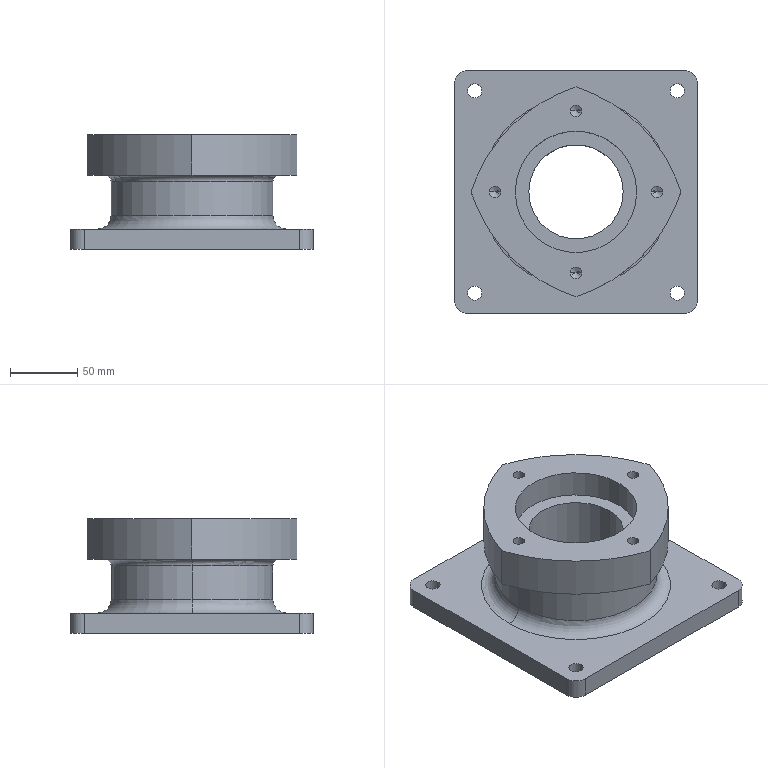Part | SolidWorks | features ICE 4, Fillet 2, 3DProfileFeature 1, CirPattern 1, Extrusion 1, HoleWzd 1 | 1 solid | 51 faces | box 180 x 180 x 85 mm | volume 1041607 mm3 | cylinder 30 | plane 9 | cone 8 | torus 4 | commonest cylinder face diameters 8.5 x8 10.5 x8 20 x4 240 x4 70 x2 90 x2
STEP:
#1=CARTESIAN_POINT('',(-45.,0.,65.));
#2=VERTEX_POINT('',#1);
#3=CARTESIAN_POINT('',(45.,0.,65.));
#4=VERTEX_POINT('',#3);
#5=CARTESIAN_POINT('',(0.,0.,65.));
#6=DIRECTION('',(0.,0.,1.));
#7=DIRECTION('',(1.,0.,0.));
#8=AXIS2_PLACEMENT_3D('',#5,#6,#7);
#9=CIRCLE('',#8,45.);
#10=EDGE_CURVE('',#2,#4,#9,.T.);
#11=ORIENTED_EDGE('',*,*,#10,.F.);
#12=CARTESIAN_POINT('',(-45.,0.,85.));
#13=VERTEX_POINT('',#12);
#14=CARTESIAN_POINT('',(-45.,0.,65.));
#15=DIRECTION('',(0.,0.,1.));
#16=VECTOR('',#15,1000.);
#17=LINE('',#14,#16);
#18=EDGE_CURVE('',#2,#13,#17,.T.);
#19=ORIENTED_EDGE('',*,*,#18,.T.);
#20=CARTESIAN_POINT('',(45.,0.,85.));
#21=VERTEX_POINT('',#20);
#22=CARTESIAN_POINT('',(0.,0.,85.));
#23=DIRECTION('',(0.,0.,1.));
#24=DIRECTION('',(1.,0.,0.));
#25=AXIS2_PLACEMENT_3D('',#22,#23,#24);
#26=CIRCLE('',#25,45.);
#27=EDGE_CURVE('',#13,#21,#26,.T.);
#28=ORIENTED_EDGE('',*,*,#27,.T.);
#29=CARTESIAN_POINT('',(45.,0.,65.));
#30=DIRECTION('',(0.,0.,1.));
#31=VECTOR('',#30,1000.);
#32=LINE('',#29,#31);
#33=EDGE_CURVE('',#4,#21,#32,.T.);
#34=ORIENTED_EDGE('',*,*,#33,.F.);
#35=EDGE_LOOP('',(#11,#19,#28,#34));
#36=FACE_OUTER_BOUND('',#35,.T.);
#37=CARTESIAN_POINT('',(0.,0.,65.));
#38=DIRECTION('',(0.,0.,1.));
#39=DIRECTION('',(1.,0.,0.));
#40=AXIS2_PLACEMENT_3D('',#37,#38,#39);
#41=CYLINDRICAL_SURFACE('',#40,45.);
#42=ADVANCED_FACE('',(#36),#41,.F.);
#43=CARTESIAN_POINT('',(-65.,0.,55.));
#44=VERTEX_POINT('',#43);
#45=CARTESIAN_POINT('',(65.,0.,55.));
#46=VERTEX_POINT('',#45);
#47=CARTESIAN_POINT('',(0.,0.,55.));
#48=DIRECTION('',(0.,0.,1.));
#49=DIRECTION('',(1.,0.,0.));
#50=AXIS2_PLACEMENT_3D('',#47,#48,#49);
#51=CIRCLE('',#50,65.);
#52=EDGE_CURVE('',#44,#46,#51,.T.);
#53=ORIENTED_EDGE('',*,*,#52,.F.);
#54=CARTESIAN_POINT('',(-60.,0.,50.));
#55=VERTEX_POINT('',#54);
#56=CARTESIAN_POINT('',(-65.,0.,50.));
#57=DIRECTION('',(0.,1.,0.));
#58=DIRECTION('',(-1.,0.,0.));
#59=AXIS2_PLACEMENT_3D('',#56,#57,#58);
#60=CIRCLE('',#59,5.);
#61=EDGE_CURVE('',#44,#55,#60,.T.);
#62=ORIENTED_EDGE('',*,*,#61,.T.);
#63=CARTESIAN_POINT('',(60.,0.,50.));
#64=VERTEX_POINT('',#63);
#65=CARTESIAN_POINT('',(0.,0.,50.));
#66=DIRECTION('',(0.,0.,-1.));
#67=DIRECTION('',(1.,0.,0.));
#68=AXIS2_PLACEMENT_3D('',#65,#66,#67);
#69=CIRCLE('',#68,60.);
#70=EDGE_CURVE('',#64,#55,#69,.T.);
#71=ORIENTED_EDGE('',*,*,#70,.F.);
#72=CARTESIAN_POINT('',(65.,0.,50.));
#73=DIRECTION('',(0.,-1.,0.));
#74=DIRECTION('',(0.,0.,-1.));
#75=AXIS2_PLACEMENT_3D('',#72,#73,#74);
#76=CIRCLE('',#75,5.);
#77=EDGE_CURVE('',#46,#64,#76,.T.);
#78=ORIENTED_EDGE('',*,*,#77,.F.);
#79=EDGE_LOOP('',(#53,#62,#71,#78));
#80=FACE_OUTER_BOUND('',#79,.T.);
#81=CARTESIAN_POINT('',(0.,0.,50.));
#82=DIRECTION('',(0.,0.,1.));
#83=DIRECTION('',(1.,0.,0.));
#84=AXIS2_PLACEMENT_3D('',#81,#82,#83);
#85=TOROIDAL_SURFACE('',#84,65.,5.);
#86=ADVANCED_FACE('',(#80),#85,.F.);
#87=CARTESIAN_POINT('',(-60.,0.,25.));
#88=VERTEX_POINT('',#87);
#89=CARTESIAN_POINT('',(60.,0.,25.));
#90=VERTEX_POINT('',#89);
#91=CARTESIAN_POINT('',(0.,0.,25.));
#92=DIRECTION('',(0.,0.,1.));
#93=DIRECTION('',(1.,0.,0.));
#94=AXIS2_PLACEMENT_3D('',#91,#92,#93);
#95=CIRCLE('',#94,60.);
#96=EDGE_CURVE('',#88,#90,#95,.T.);
#97=ORIENTED_EDGE('',*,*,#96,.F.);
#98=CARTESIAN_POINT('',(-70.,0.,15.));
#99=VERTEX_POINT('',#98);
#100=CARTESIAN_POINT('',(-70.,0.,25.));
#101=DIRECTION('',(0.,1.,0.));
#102=DIRECTION('',(-1.,0.,0.));
#103=AXIS2_PLACEMENT_3D('',#100,#101,#102);
#104=CIRCLE('',#103,10.);
#105=EDGE_CURVE('',#88,#99,#104,.T.);
#106=ORIENTED_EDGE('',*,*,#105,.T.);
#107=CARTESIAN_POINT('',(70.,0.,15.));
#108=VERTEX_POINT('',#107);
#109=CARTESIAN_POINT('',(0.,0.,15.));
#110=DIRECTION('',(0.,0.,-1.));
#111=DIRECTION('',(1.,0.,0.));
#112=AXIS2_PLACEMENT_3D('',#109,#110,#111);
#113=CIRCLE('',#112,70.);
#114=EDGE_CURVE('',#108,#99,#113,.T.);
#115=ORIENTED_EDGE('',*,*,#114,.F.);
#116=CARTESIAN_POINT('',(70.,0.,25.));
#117=DIRECTION('',(0.,-1.,0.));
#118=DIRECTION('',(0.,0.,-1.));
#119=AXIS2_PLACEMENT_3D('',#116,#117,#118);
#120=CIRCLE('',#119,10.);
#121=EDGE_CURVE('',#90,#108,#120,.T.);
#122=ORIENTED_EDGE('',*,*,#121,.F.);
#123=EDGE_LOOP('',(#97,#106,#115,#122));
#124=FACE_OUTER_BOUND('',#123,.T.);
#125=CARTESIAN_POINT('',(0.,0.,25.));
#126=DIRECTION('',(0.,0.,1.));
#127=DIRECTION('',(1.,0.,0.));
#128=AXIS2_PLACEMENT_3D('',#125,#126,#127);
#129=TOROIDAL_SURFACE('',#128,70.,10.);
#130=ADVANCED_FACE('',(#124),#129,.F.);
#131=CARTESIAN_POINT('',(-64.25,0.,63.));
#132=VERTEX_POINT('',#131);
#133=CARTESIAN_POINT('',(-55.75,0.,63.));
#134=VERTEX_POINT('',#133);
#135=CARTESIAN_POINT('',(-60.,0.,63.));
#136=DIRECTION('',(0.,0.,1.));
#137=DIRECTION('',(1.,0.,0.));
#138=AXIS2_PLACEMENT_3D('',#135,#136,#137);
#139=CIRCLE('',#138,4.25);
#140=EDGE_CURVE('',#132,#134,#139,.T.);
#141=ORIENTED_EDGE('',*,*,#140,.F.);
#142=CARTESIAN_POINT('',(-64.25,0.,85.));
#143=VERTEX_POINT('',#142);
#144=CARTESIAN_POINT('',(-64.25,0.,85.));
#145=DIRECTION('',(0.,0.,1.));
#146=VECTOR('',#145,1000.);
#147=LINE('',#144,#146);
#148=EDGE_CURVE('',#132,#143,#147,.T.);
#149=ORIENTED_EDGE('',*,*,#148,.T.);
#150=CARTESIAN_POINT('',(-55.75,0.,85.));
#151=VERTEX_POINT('',#150);
#152=CARTESIAN_POINT('',(-60.,0.,85.));
#153=DIRECTION('',(0.,0.,1.));
#154=DIRECTION('',(1.,0.,0.));
#155=AXIS2_PLACEMENT_3D('',#152,#153,#154);
#156=CIRCLE('',#155,4.25);
#157=EDGE_CURVE('',#143,#151,#156,.T.);
#158=ORIENTED_EDGE('',*,*,#157,.T.);
#159=CARTESIAN_POINT('',(-55.75,0.,85.));
#160=DIRECTION('',(0.,0.,1.));
#161=VECTOR('',#160,1000.);
#162=LINE('',#159,#161);
#163=EDGE_CURVE('',#134,#151,#162,.T.);
#164=ORIENTED_EDGE('',*,*,#163,.F.);
#165=EDGE_LOOP('',(#141,#149,#158,#164));
#166=FACE_OUTER_BOUND('',#165,.T.);
#167=CARTESIAN_POINT('',(-60.,0.,85.));
#168=DIRECTION('',(0.,0.,1.));
#169=DIRECTION('',(1.,0.,0.));
#170=AXIS2_PLACEMENT_3D('',#167,#168,#169);
#171=CYLINDRICAL_SURFACE('',#170,4.25);
#172=ADVANCED_FACE('',(#166),#171,.F.);
#173=CARTESIAN_POINT('',(-60.,0.,60.446));
#174=VERTEX_POINT('',#173);
#175=CARTESIAN_POINT('',(-55.75,0.,63.));
#176=DIRECTION('',(0.8572,0.,0.515));
#177=VECTOR('',#176,1000.);
#178=LINE('',#175,#177);
#179=EDGE_CURVE('',#174,#134,#178,.T.);
#180=ORIENTED_EDGE('',*,*,#179,.F.);
#181=CARTESIAN_POINT('',(-64.25,0.,63.));
#182=DIRECTION('',(-0.8572,0.,0.515));
#183=VECTOR('',#182,1000.);
#184=LINE('',#181,#183);
#185=EDGE_CURVE('',#174,#132,#184,.T.);
#186=ORIENTED_EDGE('',*,*,#185,.T.);
#187=ORIENTED_EDGE('',*,*,#140,.T.);
#188=EDGE_LOOP('',(#180,#186,#187));
#189=FACE_OUTER_BOUND('',#188,.T.);
#190=CARTESIAN_POINT('',(-60.,0.,63.));
#191=DIRECTION('',(0.,0.,1.));
#192=DIRECTION('',(1.,0.,0.));
#193=AXIS2_PLACEMENT_3D('',#190,#191,#192);
#194=CONICAL_SURFACE('',#193,4.25,1.03);
#195=ADVANCED_FACE('',(#189),#194,.F.);
#196=CARTESIAN_POINT('',(-4.25,-60.,63.));
#197=VERTEX_POINT('',#196);
#198=CARTESIAN_POINT('',(4.25,-60.,63.));
#199=VERTEX_POINT('',#198);
#200=CARTESIAN_POINT('',(0.,-60.,63.));
#201=DIRECTION('',(0.,0.,1.));
#202=DIRECTION('',(1.,0.,0.));
#203=AXIS2_PLACEMENT_3D('',#200,#201,#202);
#204=CIRCLE('',#203,4.25);
#205=EDGE_CURVE('',#197,#199,#204,.T.);
#206=ORIENTED_EDGE('',*,*,#205,.F.);
#207=CARTESIAN_POINT('',(-4.25,-60.,85.));
#208=VERTEX_POINT('',#207);
#209=CARTESIAN_POINT('',(-4.25,-60.,85.));
#210=DIRECTION('',(0.,0.,1.));
#211=VECTOR('',#210,1000.);
#212=LINE('',#209,#211);
#213=EDGE_CURVE('',#197,#208,#212,.T.);
#214=ORIENTED_EDGE('',*,*,#213,.T.);
#215=CARTESIAN_POINT('',(4.25,-60.,85.));
#216=VERTEX_POINT('',#215);
#217=CARTESIAN_POINT('',(0.,-60.,85.));
#218=DIRECTION('',(0.,0.,1.));
#219=DIRECTION('',(1.,0.,0.));
#220=AXIS2_PLACEMENT_3D('',#217,#218,#219);
#221=CIRCLE('',#220,4.25);
#222=EDGE_CURVE('',#208,#216,#221,.T.);
#223=ORIENTED_EDGE('',*,*,#222,.T.);
#224=CARTESIAN_POINT('',(4.25,-60.,85.));
#225=DIRECTION('',(0.,0.,1.));
#226=VECTOR('',#225,1000.);
#227=LINE('',#224,#226);
#228=EDGE_CURVE('',#199,#216,#227,.T.);
#229=ORIENTED_EDGE('',*,*,#228,.F.);
#230=EDGE_LOOP('',(#206,#214,#223,#229));
#231=FACE_OUTER_BOUND('',#230,.T.);
#232=CARTESIAN_POINT('',(0.,-60.,85.));
#233=DIRECTION('',(0.,0.,1.));
#234=DIRECTION('',(1.,0.,0.));
#235=AXIS2_PLACEMENT_3D('',#232,#233,#234);
#236=CYLINDRICAL_SURFACE('',#235,4.25);
#237=ADVANCED_FACE('',(#231),#236,.F.);
#238=CARTESIAN_POINT('',(0.,-60.,60.446));
#239=VERTEX_POINT('',#238);
#240=CARTESIAN_POINT('',(4.25,-60.,63.));
#241=DIRECTION('',(0.8572,0.,0.515));
#242=VECTOR('',#241,1000.);
#243=LINE('',#240,#242);
#244=EDGE_CURVE('',#239,#199,#243,.T.);
#245=ORIENTED_EDGE('',*,*,#244,.F.);
#246=CARTESIAN_POINT('',(-4.25,-60.,63.));
#247=DIRECTION('',(-0.8572,0.,0.515));
#248=VECTOR('',#247,1000.);
#249=LINE('',#246,#248);
#250=EDGE_CURVE('',#239,#197,#249,.T.);
#251=ORIENTED_EDGE('',*,*,#250,.T.);
#252=ORIENTED_EDGE('',*,*,#205,.T.);
#253=EDGE_LOOP('',(#245,#251,#252));
#254=FACE_OUTER_BOUND('',#253,.T.);
#255=CARTESIAN_POINT('',(0.,-60.,63.));
#256=DIRECTION('',(0.,0.,1.));
#257=DIRECTION('',(1.,0.,0.));
#258=AXIS2_PLACEMENT_3D('',#255,#256,#257);
#259=CONICAL_SURFACE('',#258,4.25,1.03);
#260=ADVANCED_FACE('',(#254),#259,.F.);
#261=CARTESIAN_POINT('',(55.75,0.,63.));
#262=VERTEX_POINT('',#261);
#263=CARTESIAN_POINT('',(64.25,0.,63.));
#264=VERTEX_POINT('',#263);
#265=CARTESIAN_POINT('',(60.,0.,63.));
#266=DIRECTION('',(0.,0.,1.));
#267=DIRECTION('',(1.,0.,0.));
#268=AXIS2_PLACEMENT_3D('',#265,#266,#267);
#269=CIRCLE('',#268,4.25);
#270=EDGE_CURVE('',#262,#264,#269,.T.);
#271=ORIENTED_EDGE('',*,*,#270,.F.);
#272=CARTESIAN_POINT('',(55.75,0.,85.));
#273=VERTEX_POINT('',#272);
#274=CARTESIAN_POINT('',(55.75,0.,85.));
#275=DIRECTION('',(0.,0.,1.));
#276=VECTOR('',#275,1000.);
#277=LINE('',#274,#276);
#278=EDGE_CURVE('',#262,#273,#277,.T.);
#279=ORIENTED_EDGE('',*,*,#278,.T.);
#280=CARTESIAN_POINT('',(64.25,0.,85.));
#281=VERTEX_POINT('',#280);
#282=CARTESIAN_POINT('',(60.,0.,85.));
#283=DIRECTION('',(0.,0.,1.));
#284=DIRECTION('',(1.,0.,0.));
#285=AXIS2_PLACEMENT_3D('',#282,#283,#284);
#286=CIRCLE('',#285,4.25);
#287=EDGE_CURVE('',#273,#281,#286,.T.);
#288=ORIENTED_EDGE('',*,*,#287,.T.);
#289=CARTESIAN_POINT('',(64.25,0.,85.));
#290=DIRECTION('',(0.,0.,1.));
#291=VECTOR('',#290,1000.);
#292=LINE('',#289,#291);
#293=EDGE_CURVE('',#264,#281,#292,.T.);
#294=ORIENTED_EDGE('',*,*,#293,.F.);
#295=EDGE_LOOP('',(#271,#279,#288,#294));
#296=FACE_OUTER_BOUND('',#295,.T.);
#297=CARTESIAN_POINT('',(60.,0.,85.));
#298=DIRECTION('',(0.,0.,1.));
#299=DIRECTION('',(1.,0.,0.));
#300=AXIS2_PLACEMENT_3D('',#297,#298,#299);
#301=CYLINDRICAL_SURFACE('',#300,4.25);
#302=ADVANCED_FACE('',(#296),#301,.F.);
#303=CARTESIAN_POINT('',(60.,0.,60.446));
#304=VERTEX_POINT('',#303);
#305=CARTESIAN_POINT('',(64.25,0.,63.));
#306=DIRECTION('',(0.8572,0.,0.515));
#307=VECTOR('',#306,1000.);
#308=LINE('',#305,#307);
#309=EDGE_CURVE('',#304,#264,#308,.T.);
#310=ORIENTED_EDGE('',*,*,#309,.F.);
#311=CARTESIAN_POINT('',(55.75,0.,63.));
#312=DIRECTION('',(-0.8572,0.,0.515));
#313=VECTOR('',#312,1000.);
#314=LINE('',#311,#313);
#315=EDGE_CURVE('',#304,#262,#314,.T.);
#316=ORIENTED_EDGE('',*,*,#315,.T.);
#317=ORIENTED_EDGE('',*,*,#270,.T.);
#318=EDGE_LOOP('',(#310,#316,#317));
#319=FACE_OUTER_BOUND('',#318,.T.);
#320=CARTESIAN_POINT('',(60.,0.,63.));
#321=DIRECTION('',(0.,0.,1.));
#322=DIRECTION('',(1.,0.,0.));
#323=AXIS2_PLACEMENT_3D('',#320,#321,#322);
#324=CONICAL_SURFACE('',#323,4.25,1.03);
#325=ADVANCED_FACE('',(#319),#324,.F.);
#326=CARTESIAN_POINT('',(-4.25,60.,63.));
#327=VERTEX_POINT('',#326);
#328=CARTESIAN_POINT('',(4.25,60.,63.));
#329=VERTEX_POINT('',#328);
#330=CARTESIAN_POINT('',(0.,60.,63.));
#331=DIRECTION('',(0.,0.,1.));
#332=DIRECTION('',(1.,0.,0.));
#333=AXIS2_PLACEMENT_3D('',#330,#331,#332);
#334=CIRCLE('',#333,4.25);
#335=EDGE_CURVE('',#327,#329,#334,.T.);
#336=ORIENTED_EDGE('',*,*,#335,.F.);
#337=CARTESIAN_POINT('',(-4.25,60.,85.));
#338=VERTEX_POINT('',#337);
#339=CARTESIAN_POINT('',(-4.25,60.,85.));
#340=DIRECTION('',(0.,0.,1.));
#341=VECTOR('',#340,1000.);
#342=LINE('',#339,#341);
#343=EDGE_CURVE('',#327,#338,#342,.T.);
#344=ORIENTED_EDGE('',*,*,#343,.T.);
#345=CARTESIAN_POINT('',(4.25,60.,85.));
#346=VERTEX_POINT('',#345);
#347=CARTESIAN_POINT('',(0.,60.,85.));
#348=DIRECTION('',(0.,0.,1.));
#349=DIRECTION('',(1.,0.,0.));
#350=AXIS2_PLACEMENT_3D('',#347,#348,#349);
#351=CIRCLE('',#350,4.25);
#352=EDGE_CURVE('',#338,#346,#351,.T.);
#353=ORIENTED_EDGE('',*,*,#352,.T.);
#354=CARTESIAN_POINT('',(4.25,60.,85.));
#355=DIRECTION('',(0.,0.,1.));
#356=VECTOR('',#355,1000.);
#357=LINE('',#354,#356);
#358=EDGE_CURVE('',#329,#346,#357,.T.);
#359=ORIENTED_EDGE('',*,*,#358,.F.);
#360=EDGE_LOOP('',(#336,#344,#353,#359));
#361=FACE_OUTER_BOUND('',#360,.T.);
#362=CARTESIAN_POINT('',(0.,60.,85.));
#363=DIRECTION('',(0.,0.,1.));
#364=DIRECTION('',(1.,0.,0.));
#365=AXIS2_PLACEMENT_3D('',#362,#363,#364);
#366=CYLINDRICAL_SURFACE('',#365,4.25);
#367=ADVANCED_FACE('',(#361),#366,.F.);
#368=CARTESIAN_POINT('',(0.,60.,60.446));
#369=VERTEX_POINT('',#368);
#370=CARTESIAN_POINT('',(4.25,60.,63.));
#371=DIRECTION('',(0.8572,0.,0.515));
#372=VECTOR('',#371,1000.);
#373=LINE('',#370,#372);
#374=EDGE_CURVE('',#369,#329,#373,.T.);
#375=ORIENTED_EDGE('',*,*,#374,.F.);
#376=CARTESIAN_POINT('',(-4.25,60.,63.));
#377=DIRECTION('',(-0.8572,0.,0.515));
#378=VECTOR('',#377,1000.);
#379=LINE('',#376,#378);
#380=EDGE_CURVE('',#369,#327,#379,.T.);
#381=ORIENTED_EDGE('',*,*,#380,.T.);
#382=ORIENTED_EDGE('',*,*,#335,.T.);
#383=EDGE_LOOP('',(#375,#381,#382));
#384=FACE_OUTER_BOUND('',#383,.T.);
#385=CARTESIAN_POINT('',(0.,60.,63.));
#386=DIRECTION('',(0.,0.,1.));
#387=DIRECTION('',(1.,0.,0.));
#388=AXIS2_PLACEMENT_3D('',#385,#386,#387);
#389=CONICAL_SURFACE('',#388,4.25,1.03);
#390=ADVANCED_FACE('',(#384),#389,.F.);
#391=CARTESIAN_POINT('',(0.,0.,50.));
#392=DIRECTION('',(0.,0.,-1.));
#393=DIRECTION('',(1.,0.,0.));
#394=AXIS2_PLACEMENT_3D('',#391,#392,#393);
#395=CIRCLE('',#394,60.);
#396=EDGE_CURVE('',#55,#64,#395,.T.);
#397=ORIENTED_EDGE('',*,*,#396,.T.);
#398=CARTESIAN_POINT('',(60.,0.,55.));
#399=DIRECTION('',(0.,0.,-1.));
#400=VECTOR('',#399,1000.);
#401=LINE('',#398,#400);
#402=EDGE_CURVE('',#64,#90,#401,.T.);
#403=ORIENTED_EDGE('',*,*,#402,.T.);
#404=CARTESIAN_POINT('',(0.,0.,25.));
#405=DIRECTION('',(0.,0.,1.));
#406=DIRECTION('',(1.,0.,0.));
#407=AXIS2_PLACEMENT_3D('',#404,#405,#406);
#408=CIRCLE('',#407,60.);
#409=EDGE_CURVE('',#90,#88,#408,.T.);
#410=ORIENTED_EDGE('',*,*,#409,.T.);
#411=CARTESIAN_POINT('',(-60.,0.,55.));
#412=DIRECTION('',(0.,0.,-1.));
#413=VECTOR('',#412,1000.);
#414=LINE('',#411,#413);
#415=EDGE_CURVE('',#55,#88,#414,.T.);
#416=ORIENTED_EDGE('',*,*,#415,.F.);
#417=EDGE_LOOP('',(#397,#403,#410,#416));
#418=FACE_OUTER_BOUND('',#417,.T.);
#419=CARTESIAN_POINT('',(0.,0.,55.));
#420=DIRECTION('',(0.,0.,-1.));
#421=DIRECTION('',(-1.,0.,0.));
#422=AXIS2_PLACEMENT_3D('',#419,#420,#421);
#423=CYLINDRICAL_SURFACE('',#422,60.);
#424=ADVANCED_FACE('',(#418),#423,.T.);
#425=CARTESIAN_POINT('',(69.75,-75.,15.));
#426=VERTEX_POINT('',#425);
#427=CARTESIAN_POINT('',(80.25,-75.,15.));
#428=VERTEX_POINT('',#427);
#429=CARTESIAN_POINT('',(75.,-75.,15.));
#430=DIRECTION('',(0.,0.,1.));
#431=DIRECTION('',(1.,0.,0.));
#432=AXIS2_PLACEMENT_3D('',#429,#430,#431);
#433=CIRCLE('',#432,5.25);
#434=EDGE_CURVE('',#426,#428,#433,.T.);
#435=ORIENTED_EDGE('',*,*,#434,.T.);
#436=CARTESIAN_POINT('',(80.25,-75.,0.));
#437=VERTEX_POINT('',#436);
#438=CARTESIAN_POINT('',(80.25,-75.,15.));
#439=DIRECTION('',(0.,0.,-1.));
#440=VECTOR('',#439,1000.);
#441=LINE('',#438,#440);
#442=EDGE_CURVE('',#428,#437,#441,.T.);
#443=ORIENTED_EDGE('',*,*,#442,.T.);
#444=CARTESIAN_POINT('',(69.75,-75.,0.));
#445=VERTEX_POINT('',#444);
#446=CARTESIAN_POINT('',(75.,-75.,0.));
#447=DIRECTION('',(0.,0.,1.));
#448=DIRECTION('',(1.,0.,0.));
#449=AXIS2_PLACEMENT_3D('',#446,#447,#448);
#450=CIRCLE('',#449,5.25);
#451=EDGE_CURVE('',#445,#437,#450,.T.);
#452=ORIENTED_EDGE('',*,*,#451,.F.);
#453=CARTESIAN_POINT('',(69.75,-75.,15.));
#454=DIRECTION('',(0.,0.,-1.));
#455=VECTOR('',#454,1000.);
#456=LINE('',#453,#455);
#457=EDGE_CURVE('',#426,#445,#456,.T.);
#458=ORIENTED_EDGE('',*,*,#457,.F.);
#459=EDGE_LOOP('',(#435,#443,#452,#458));
#460=FACE_OUTER_BOUND('',#459,.T.);
#461=CARTESIAN_POINT('',(75.,-75.,15.));
#462=DIRECTION('',(0.,0.,-1.));
#463=DIRECTION('',(-1.,0.,0.));
#464=AXIS2_PLACEMENT_3D('',#461,#462,#463);
#465=CYLINDRICAL_SURFACE('',#464,5.25);
#466=ADVANCED_FACE('',(#460),#465,.F.);
#467=CARTESIAN_POINT('',(-80.25,-75.,15.));
#468=VERTEX_POINT('',#467);
#469=CARTESIAN_POINT('',(-69.75,-75.,15.));
#470=VERTEX_POINT('',#469);
#471=CARTESIAN_POINT('',(-75.,-75.,15.));
#472=DIRECTION('',(0.,0.,1.));
#473=DIRECTION('',(1.,0.,0.));
#474=AXIS2_PLACEMENT_3D('',#471,#472,#473);
#475=CIRCLE('',#474,5.25);
#476=EDGE_CURVE('',#468,#470,#475,.T.);
#477=ORIENTED_EDGE('',*,*,#476,.T.);
#478=CARTESIAN_POINT('',(-69.75,-75.,0.));
#479=VERTEX_POINT('',#478);
#480=CARTESIAN_POINT('',(-69.75,-75.,15.));
#481=DIRECTION('',(0.,0.,-1.));
#482=VECTOR('',#481,1000.);
#483=LINE('',#480,#482);
#484=EDGE_CURVE('',#470,#479,#483,.T.);
#485=ORIENTED_EDGE('',*,*,#484,.T.);
#486=CARTESIAN_POINT('',(-80.25,-75.,0.));
#487=VERTEX_POINT('',#486);
#488=CARTESIAN_POINT('',(-75.,-75.,0.));
#489=DIRECTION('',(0.,0.,1.));
#490=DIRECTION('',(1.,0.,0.));
#491=AXIS2_PLACEMENT_3D('',#488,#489,#490);
#492=CIRCLE('',#491,5.25);
#493=EDGE_CURVE('',#487,#479,#492,.T.);
#494=ORIENTED_EDGE('',*,*,#493,.F.);
#495=CARTESIAN_POINT('',(-80.25,-75.,15.));
#496=DIRECTION('',(0.,0.,-1.));
#497=VECTOR('',#496,1000.);
#498=LINE('',#495,#497);
#499=EDGE_CURVE('',#468,#487,#498,.T.);
#500=ORIENTED_EDGE('',*,*,#499,.F.);
#501=EDGE_LOOP('',(#477,#485,#494,#500));
#502=FACE_OUTER_BOUND('',#501,.T.);
#503=CARTESIAN_POINT('',(-75.,-75.,15.));
#504=DIRECTION('',(0.,0.,-1.));
#505=DIRECTION('',(-1.,0.,0.));
#506=AXIS2_PLACEMENT_3D('',#503,#504,#505);
#507=CYLINDRICAL_SURFACE('',#506,5.25);
#508=ADVANCED_FACE('',(#502),#507,.F.);
#509=CARTESIAN_POINT('',(69.75,75.,15.));
#510=VERTEX_POINT('',#509);
#511=CARTESIAN_POINT('',(80.25,75.,15.));
#512=VERTEX_POINT('',#511);
#513=CARTESIAN_POINT('',(75.,75.,15.));
#514=DIRECTION('',(0.,0.,1.));
#515=DIRECTION('',(1.,0.,0.));
#516=AXIS2_PLACEMENT_3D('',#513,#514,#515);
#517=CIRCLE('',#516,5.25);
#518=EDGE_CURVE('',#510,#512,#517,.T.);
#519=ORIENTED_EDGE('',*,*,#518,.T.);
#520=CARTESIAN_POINT('',(80.25,75.,0.));
#521=VERTEX_POINT('',#520);
#522=CARTESIAN_POINT('',(80.25,75.,15.));
#523=DIRECTION('',(0.,0.,-1.));
#524=VECTOR('',#523,1000.);
#525=LINE('',#522,#524);
#526=EDGE_CURVE('',#512,#521,#525,.T.);
#527=ORIENTED_EDGE('',*,*,#526,.T.);
#528=CARTESIAN_POINT('',(69.75,75.,0.));
#529=VERTEX_POINT('',#528);
#530=CARTESIAN_POINT('',(75.,75.,0.));
#531=DIRECTION('',(0.,0.,1.));
#532=DIRECTION('',(1.,0.,0.));
#533=AXIS2_PLACEMENT_3D('',#530,#531,#532);
#534=CIRCLE('',#533,5.25);
#535=EDGE_CURVE('',#529,#521,#534,.T.);
#536=ORIENTED_EDGE('',*,*,#535,.F.);
#537=CARTESIAN_POINT('',(69.75,75.,15.));
#538=DIRECTION('',(0.,0.,-1.));
#539=VECTOR('',#538,1000.);
#540=LINE('',#537,#539);
#541=EDGE_CURVE('',#510,#529,#540,.T.);
#542=ORIENTED_EDGE('',*,*,#541,.F.);
#543=EDGE_LOOP('',(#519,#527,#536,#542));
#544=FACE_OUTER_BOUND('',#543,.T.);
#545=CARTESIAN_POINT('',(75.,75.,15.));
#546=DIRECTION('',(0.,0.,-1.));
#547=DIRECTION('',(-1.,0.,0.));
#548=AXIS2_PLACEMENT_3D('',#545,#546,#547);
#549=CYLINDRICAL_SURFACE('',#548,5.25);
#550=ADVANCED_FACE('',(#544),#549,.F.);
#551=CARTESIAN_POINT('',(-80.25,75.,15.));
#552=VERTEX_POINT('',#551);
#553=CARTESIAN_POINT('',(-69.75,75.,15.));
#554=VERTEX_POINT('',#553);
#555=CARTESIAN_POINT('',(-75.,75.,15.));
#556=DIRECTION('',(0.,0.,1.));
#557=DIRECTION('',(1.,0.,0.));
#558=AXIS2_PLACEMENT_3D('',#555,#556,#557);
#559=CIRCLE('',#558,5.25);
#560=EDGE_CURVE('',#552,#554,#559,.T.);
#561=ORIENTED_EDGE('',*,*,#560,.T.);
#562=CARTESIAN_POINT('',(-69.75,75.,0.));
#563=VERTEX_POINT('',#562);
#564=CARTESIAN_POINT('',(-69.75,75.,15.));
#565=DIRECTION('',(0.,0.,-1.));
#566=VECTOR('',#565,1000.);
#567=LINE('',#564,#566);
#568=EDGE_CURVE('',#554,#563,#567,.T.);
#569=ORIENTED_EDGE('',*,*,#568,.T.);
#570=CARTESIAN_POINT('',(-80.25,75.,0.));
#571=VERTEX_POINT('',#570);
#572=CARTESIAN_POINT('',(-75.,75.,0.));
#573=DIRECTION('',(0.,0.,1.));
#574=DIRECTION('',(1.,0.,0.));
#575=AXIS2_PLACEMENT_3D('',#572,#573,#574);
#576=CIRCLE('',#575,5.25);
#577=EDGE_CURVE('',#571,#563,#576,.T.);
#578=ORIENTED_EDGE('',*,*,#577,.F.);
#579=CARTESIAN_POINT('',(-80.25,75.,15.));
#580=DIRECTION('',(0.,0.,-1.));
#581=VECTOR('',#580,1000.);
#582=LINE('',#579,#581);
#583=EDGE_CURVE('',#552,#571,#582,.T.);
#584=ORIENTED_EDGE('',*,*,#583,.F.);
#585=EDGE_LOOP('',(#561,#569,#578,#584));
#586=FACE_OUTER_BOUND('',#585,.T.);
#587=CARTESIAN_POINT('',(-75.,75.,15.));
#588=DIRECTION('',(0.,0.,-1.));
#589=DIRECTION('',(-1.,0.,0.));
#590=AXIS2_PLACEMENT_3D('',#587,#588,#589);
#591=CYLINDRICAL_SURFACE('',#590,5.25);
#592=ADVANCED_FACE('',(#586),#591,.F.);
#593=CARTESIAN_POINT('',(-35.,0.,0.));
#594=VERTEX_POINT('',#593);
#595=CARTESIAN_POINT('',(35.,0.,0.));
#596=VERTEX_POINT('',#595);
#597=CARTESIAN_POINT('',(0.,0.,0.));
#598=DIRECTION('',(0.,0.,1.));
#599=DIRECTION('',(1.,0.,0.));
#600=AXIS2_PLACEMENT_3D('',#597,#598,#599);
#601=CIRCLE('',#600,35.);
#602=EDGE_CURVE('',#594,#596,#601,.T.);
#603=ORIENTED_EDGE('',*,*,#602,.F.);
#604=CARTESIAN_POINT('',(-35.,0.,65.));
#605=VERTEX_POINT('',#604);
#606=CARTESIAN_POINT('',(-35.,0.,0.));
#607=DIRECTION('',(0.,0.,1.));
#608=VECTOR('',#607,1000.);
#609=LINE('',#606,#608);
#610=EDGE_CURVE('',#594,#605,#609,.T.);
#611=ORIENTED_EDGE('',*,*,#610,.T.);
#612=CARTESIAN_POINT('',(35.,0.,65.));
#613=VERTEX_POINT('',#612);
#614=CARTESIAN_POINT('',(0.,0.,65.));
#615=DIRECTION('',(0.,0.,-1.));
#616=DIRECTION('',(1.,0.,0.));
#617=AXIS2_PLACEMENT_3D('',#614,#615,#616);
#618=CIRCLE('',#617,35.);
#619=EDGE_CURVE('',#613,#605,#618,.T.);
#620=ORIENTED_EDGE('',*,*,#619,.F.);
#621=CARTESIAN_POINT('',(35.,0.,0.));
#622=DIRECTION('',(0.,0.,1.));
#623=VECTOR('',#622,1000.);
#624=LINE('',#621,#623);
#625=EDGE_CURVE('',#596,#613,#624,.T.);
#626=ORIENTED_EDGE('',*,*,#625,.F.);
#627=EDGE_LOOP('',(#603,#611,#620,#626));
#628=FACE_OUTER_BOUND('',#627,.T.);
#629=CARTESIAN_POINT('',(0.,0.,0.));
#630=DIRECTION('',(0.,0.,1.));
#631=DIRECTION('',(1.,0.,0.));
#632=AXIS2_PLACEMENT_3D('',#629,#630,#631);
#633=CYLINDRICAL_SURFACE('',#632,35.);
#634=ADVANCED_FACE('',(#628),#633,.F.);
#635=ORIENTED_EDGE('',*,*,#610,.F.);
#636=CARTESIAN_POINT('',(0.,0.,0.));
#637=DIRECTION('',(0.,0.,1.));
#638=DIRECTION('',(1.,0.,0.));
#639=AXIS2_PLACEMENT_3D('',#636,#637,#638);
#640=CIRCLE('',#639,35.);
#641=EDGE_CURVE('',#596,#594,#640,.T.);
#642=ORIENTED_EDGE('',*,*,#641,.F.);
#643=ORIENTED_EDGE('',*,*,#625,.T.);
#644=CARTESIAN_POINT('',(0.,0.,65.));
#645=DIRECTION('',(0.,0.,-1.));
#646=DIRECTION('',(1.,0.,0.));
#647=AXIS2_PLACEMENT_3D('',#644,#645,#646);
#648=CIRCLE('',#647,35.);
#649=EDGE_CURVE('',#605,#613,#648,.T.);
#650=ORIENTED_EDGE('',*,*,#649,.F.);
#651=EDGE_LOOP('',(#635,#642,#643,#650));
#652=FACE_OUTER_BOUND('',#651,.T.);
#653=CARTESIAN_POINT('',(0.,0.,0.));
#654=DIRECTION('',(0.,0.,1.));
#655=DIRECTION('',(1.,0.,0.));
#656=AXIS2_PLACEMENT_3D('',#653,#654,#655);
#657=CYLINDRICAL_SURFACE('',#656,35.);
#658=ADVANCED_FACE('',(#652),#657,.F.);
#659=ORIENTED_EDGE('',*,*,#114,.T.);
#660=CARTESIAN_POINT('',(0.,0.,15.));
#661=DIRECTION('',(0.,0.,-1.));
#662=DIRECTION('',(1.,0.,0.));
#663=AXIS2_PLACEMENT_3D('',#660,#661,#662);
#664=CIRCLE('',#663,70.);
#665=EDGE_CURVE('',#99,#108,#664,.T.);
#666=ORIENTED_EDGE('',*,*,#665,.T.);
#667=EDGE_LOOP('',(#659,#666));
#668=FACE_BOUND('',#667,.T.);
#669=ORIENTED_EDGE('',*,*,#476,.F.);
#670=CARTESIAN_POINT('',(-75.,-75.,15.));
#671=DIRECTION('',(0.,0.,1.));
#672=DIRECTION('',(1.,0.,0.));
#673=AXIS2_PLACEMENT_3D('',#670,#671,#672);
#674=CIRCLE('',#673,5.25);
#675=EDGE_CURVE('',#470,#468,#674,.T.);
#676=ORIENTED_EDGE('',*,*,#675,.F.);
#677=EDGE_LOOP('',(#669,#676));
#678=FACE_BOUND('',#677,.T.);
#679=ORIENTED_EDGE('',*,*,#560,.F.);
#680=CARTESIAN_POINT('',(-75.,75.,15.));
#681=DIRECTION('',(0.,0.,1.));
#682=DIRECTION('',(1.,0.,0.));
#683=AXIS2_PLACEMENT_3D('',#680,#681,#682);
#684=CIRCLE('',#683,5.25);
#685=EDGE_CURVE('',#554,#552,#684,.T.);
#686=ORIENTED_EDGE('',*,*,#685,.F.);
#687=EDGE_LOOP('',(#679,#686));
#688=FACE_BOUND('',#687,.T.);
#689=CARTESIAN_POINT('',(-90.,-80.,15.));
#690=VERTEX_POINT('',#689);
#691=CARTESIAN_POINT('',(-80.,-90.,15.));
#692=VERTEX_POINT('',#691);
#693=CARTESIAN_POINT('',(-80.,-80.,15.));
#694=DIRECTION('',(0.,0.,1.));
#695=DIRECTION('',(1.,0.,0.));
#696=AXIS2_PLACEMENT_3D('',#693,#694,#695);
#697=CIRCLE('',#696,10.);
#698=EDGE_CURVE('',#690,#692,#697,.T.);
#699=ORIENTED_EDGE('',*,*,#698,.T.);
#700=CARTESIAN_POINT('',(80.,-90.,15.));
#701=VERTEX_POINT('',#700);
#702=CARTESIAN_POINT('',(-80.,-90.,15.));
#703=DIRECTION('',(1.,0.,0.));
#704=VECTOR('',#703,1000.);
#705=LINE('',#702,#704);
#706=EDGE_CURVE('',#692,#701,#705,.T.);
#707=ORIENTED_EDGE('',*,*,#706,.T.);
#708=CARTESIAN_POINT('',(90.,-80.,15.));
#709=VERTEX_POINT('',#708);
#710=CARTESIAN_POINT('',(80.,-80.,15.));
#711=DIRECTION('',(0.,0.,1.));
#712=DIRECTION('',(1.,0.,0.));
#713=AXIS2_PLACEMENT_3D('',#710,#711,#712);
#714=CIRCLE('',#713,10.);
#715=EDGE_CURVE('',#701,#709,#714,.T.);
#716=ORIENTED_EDGE('',*,*,#715,.T.);
#717=CARTESIAN_POINT('',(90.,80.,15.));
#718=VERTEX_POINT('',#717);
#719=CARTESIAN_POINT('',(90.,80.,15.));
#720=DIRECTION('',(0.,1.,0.));
#721=VECTOR('',#720,1000.);
#722=LINE('',#719,#721);
#723=EDGE_CURVE('',#709,#718,#722,.T.);
#724=ORIENTED_EDGE('',*,*,#723,.T.);
#725=CARTESIAN_POINT('',(80.,90.,15.));
#726=VERTEX_POINT('',#725);
#727=CARTESIAN_POINT('',(80.,80.,15.));
#728=DIRECTION('',(0.,0.,1.));
#729=DIRECTION('',(-1.,0.,0.));
#730=AXIS2_PLACEMENT_3D('',#727,#728,#729);
#731=CIRCLE('',#730,10.);
#732=EDGE_CURVE('',#718,#726,#731,.T.);
#733=ORIENTED_EDGE('',*,*,#732,.T.);
#734=CARTESIAN_POINT('',(-80.,90.,15.));
#735=VERTEX_POINT('',#734);
#736=CARTESIAN_POINT('',(-80.,90.,15.));
#737=DIRECTION('',(-1.,0.,0.));
#738=VECTOR('',#737,1000.);
#739=LINE('',#736,#738);
#740=EDGE_CURVE('',#726,#735,#739,.T.);
#741=ORIENTED_EDGE('',*,*,#740,.T.);
#742=CARTESIAN_POINT('',(-90.,80.,15.));
#743=VERTEX_POINT('',#742);
#744=CARTESIAN_POINT('',(-80.,80.,15.));
#745=DIRECTION('',(0.,0.,1.));
#746=DIRECTION('',(1.,0.,0.));
#747=AXIS2_PLACEMENT_3D('',#744,#745,#746);
#748=CIRCLE('',#747,10.);
#749=EDGE_CURVE('',#735,#743,#748,.T.);
#750=ORIENTED_EDGE('',*,*,#749,.T.);
#751=CARTESIAN_POINT('',(-90.,80.,15.));
#752=DIRECTION('',(0.,-1.,0.));
#753=VECTOR('',#752,1000.);
#754=LINE('',#751,#753);
#755=EDGE_CURVE('',#743,#690,#754,.T.);
#756=ORIENTED_EDGE('',*,*,#755,.T.);
#757=EDGE_LOOP('',(#699,#707,#716,#724,#733,#741,#750,#756));
#758=FACE_OUTER_BOUND('',#757,.T.);
#759=ORIENTED_EDGE('',*,*,#518,.F.);
#760=CARTESIAN_POINT('',(75.,75.,15.));
#761=DIRECTION('',(0.,0.,1.));
#762=DIRECTION('',(1.,0.,0.));
#763=AXIS2_PLACEMENT_3D('',#760,#761,#762);
#764=CIRCLE('',#763,5.25);
#765=EDGE_CURVE('',#512,#510,#764,.T.);
#766=ORIENTED_EDGE('',*,*,#765,.F.);
#767=EDGE_LOOP('',(#759,#766));
#768=FACE_BOUND('',#767,.T.);
#769=ORIENTED_EDGE('',*,*,#434,.F.);
#770=CARTESIAN_POINT('',(75.,-75.,15.));
#771=DIRECTION('',(0.,0.,1.));
#772=DIRECTION('',(1.,0.,0.));
#773=AXIS2_PLACEMENT_3D('',#770,#771,#772);
#774=CIRCLE('',#773,5.25);
#775=EDGE_CURVE('',#428,#426,#774,.T.);
#776=ORIENTED_EDGE('',*,*,#775,.F.);
#777=EDGE_LOOP('',(#769,#776));
#778=FACE_BOUND('',#777,.T.);
#779=CARTESIAN_POINT('',(-80.,-80.,15.));
#780=DIRECTION('',(0.,0.,1.));
#781=DIRECTION('',(1.,0.,0.));
#782=AXIS2_PLACEMENT_3D('',#779,#780,#781);
#783=PLANE('',#782);
#784=ADVANCED_FACE('',(#668,#678,#688,#758,#768,#778),#783,.T.);
#785=ORIENTED_EDGE('',*,*,#641,.T.);
#786=ORIENTED_EDGE('',*,*,#602,.T.);
#787=EDGE_LOOP('',(#785,#786));
#788=FACE_BOUND('',#787,.T.);
#789=CARTESIAN_POINT('',(-90.,-80.,0.));
#790=VERTEX_POINT('',#789);
#791=CARTESIAN_POINT('',(-80.,-90.,0.));
#792=VERTEX_POINT('',#791);
#793=CARTESIAN_POINT('',(-80.,-80.,0.));
#794=DIRECTION('',(0.,0.,1.));
#795=DIRECTION('',(1.,0.,0.));
#796=AXIS2_PLACEMENT_3D('',#793,#794,#795);
#797=CIRCLE('',#796,10.);
#798=EDGE_CURVE('',#790,#792,#797,.T.);
#799=ORIENTED_EDGE('',*,*,#798,.F.);
#800=CARTESIAN_POINT('',(-90.,80.,0.));
#801=VERTEX_POINT('',#800);
#802=CARTESIAN_POINT('',(-90.,80.,0.));
#803=DIRECTION('',(0.,-1.,0.));
#804=VECTOR('',#803,1000.);
#805=LINE('',#802,#804);
#806=EDGE_CURVE('',#801,#790,#805,.T.);
#807=ORIENTED_EDGE('',*,*,#806,.F.);
#808=CARTESIAN_POINT('',(-80.,90.,0.));
#809=VERTEX_POINT('',#808);
#810=CARTESIAN_POINT('',(-80.,80.,0.));
#811=DIRECTION('',(0.,0.,1.));
#812=DIRECTION('',(1.,0.,0.));
#813=AXIS2_PLACEMENT_3D('',#810,#811,#812);
#814=CIRCLE('',#813,10.);
#815=EDGE_CURVE('',#809,#801,#814,.T.);
#816=ORIENTED_EDGE('',*,*,#815,.F.);
#817=CARTESIAN_POINT('',(80.,90.,0.));
#818=VERTEX_POINT('',#817);
#819=CARTESIAN_POINT('',(-80.,90.,0.));
#820=DIRECTION('',(-1.,0.,0.));
#821=VECTOR('',#820,1000.);
#822=LINE('',#819,#821);
#823=EDGE_CURVE('',#818,#809,#822,.T.);
#824=ORIENTED_EDGE('',*,*,#823,.F.);
#825=CARTESIAN_POINT('',(90.,80.,0.));
#826=VERTEX_POINT('',#825);
#827=CARTESIAN_POINT('',(80.,80.,0.));
#828=DIRECTION('',(0.,0.,1.));
#829=DIRECTION('',(-1.,0.,0.));
#830=AXIS2_PLACEMENT_3D('',#827,#828,#829);
#831=CIRCLE('',#830,10.);
#832=EDGE_CURVE('',#826,#818,#831,.T.);
#833=ORIENTED_EDGE('',*,*,#832,.F.);
#834=CARTESIAN_POINT('',(90.,-80.,0.));
#835=VERTEX_POINT('',#834);
#836=CARTESIAN_POINT('',(90.,80.,0.));
#837=DIRECTION('',(0.,1.,0.));
#838=VECTOR('',#837,1000.);
#839=LINE('',#836,#838);
#840=EDGE_CURVE('',#835,#826,#839,.T.);
#841=ORIENTED_EDGE('',*,*,#840,.F.);
#842=CARTESIAN_POINT('',(80.,-90.,0.));
#843=VERTEX_POINT('',#842);
#844=CARTESIAN_POINT('',(80.,-80.,0.));
#845=DIRECTION('',(0.,0.,1.));
#846=DIRECTION('',(1.,0.,0.));
#847=AXIS2_PLACEMENT_3D('',#844,#845,#846);
#848=CIRCLE('',#847,10.);
#849=EDGE_CURVE('',#843,#835,#848,.T.);
#850=ORIENTED_EDGE('',*,*,#849,.F.);
#851=CARTESIAN_POINT('',(-80.,-90.,0.));
#852=DIRECTION('',(1.,0.,0.));
#853=VECTOR('',#852,1000.);
#854=LINE('',#851,#853);
#855=EDGE_CURVE('',#792,#843,#854,.T.);
#856=ORIENTED_EDGE('',*,*,#855,.F.);
#857=EDGE_LOOP('',(#799,#807,#816,#824,#833,#841,#850,#856));
#858=FACE_OUTER_BOUND('',#857,.T.);
#859=ORIENTED_EDGE('',*,*,#577,.T.);
#860=CARTESIAN_POINT('',(-75.,75.,0.));
#861=DIRECTION('',(0.,0.,1.));
#862=DIRECTION('',(1.,0.,0.));
#863=AXIS2_PLACEMENT_3D('',#860,#861,#862);
#864=CIRCLE('',#863,5.25);
#865=EDGE_CURVE('',#563,#571,#864,.T.);
#866=ORIENTED_EDGE('',*,*,#865,.T.);
#867=EDGE_LOOP('',(#859,#866));
#868=FACE_BOUND('',#867,.T.);
#869=ORIENTED_EDGE('',*,*,#535,.T.);
#870=CARTESIAN_POINT('',(75.,75.,0.));
#871=DIRECTION('',(0.,0.,1.));
#872=DIRECTION('',(1.,0.,0.));
#873=AXIS2_PLACEMENT_3D('',#870,#871,#872);
#874=CIRCLE('',#873,5.25);
#875=EDGE_CURVE('',#521,#529,#874,.T.);
#876=ORIENTED_EDGE('',*,*,#875,.T.);
#877=EDGE_LOOP('',(#869,#876));
#878=FACE_BOUND('',#877,.T.);
#879=ORIENTED_EDGE('',*,*,#493,.T.);
#880=CARTESIAN_POINT('',(-75.,-75.,0.));
#881=DIRECTION('',(0.,0.,1.));
#882=DIRECTION('',(1.,0.,0.));
#883=AXIS2_PLACEMENT_3D('',#880,#881,#882);
#884=CIRCLE('',#883,5.25);
#885=EDGE_CURVE('',#479,#487,#884,.T.);
#886=ORIENTED_EDGE('',*,*,#885,.T.);
#887=EDGE_LOOP('',(#879,#886));
#888=FACE_BOUND('',#887,.T.);
#889=ORIENTED_EDGE('',*,*,#451,.T.);
#890=CARTESIAN_POINT('',(75.,-75.,0.));
#891=DIRECTION('',(0.,0.,1.));
#892=DIRECTION('',(1.,0.,0.));
#893=AXIS2_PLACEMENT_3D('',#890,#891,#892);
#894=CIRCLE('',#893,5.25);
#895=EDGE_CURVE('',#437,#445,#894,.T.);
#896=ORIENTED_EDGE('',*,*,#895,.T.);
#897=EDGE_LOOP('',(#889,#896));
#898=FACE_BOUND('',#897,.T.);
#899=CARTESIAN_POINT('',(-80.,-80.,0.));
#900=DIRECTION('',(0.,0.,1.));
#901=DIRECTION('',(1.,0.,0.));
#902=AXIS2_PLACEMENT_3D('',#899,#900,#901);
#903=PLANE('',#902);
#904=ADVANCED_FACE('',(#788,#858,#868,#878,#888,#898),#903,.F.);
#905=ORIENTED_EDGE('',*,*,#798,.T.);
#906=CARTESIAN_POINT('',(-80.,-90.,15.));
#907=DIRECTION('',(0.,0.,-1.));
#908=VECTOR('',#907,1000.);
#909=LINE('',#906,#908);
#910=EDGE_CURVE('',#692,#792,#909,.T.);
#911=ORIENTED_EDGE('',*,*,#910,.F.);
#912=ORIENTED_EDGE('',*,*,#698,.F.);
#913=CARTESIAN_POINT('',(-90.,-80.,15.));
#914=DIRECTION('',(0.,0.,-1.));
#915=VECTOR('',#914,1000.);
#916=LINE('',#913,#915);
#917=EDGE_CURVE('',#690,#790,#916,.T.);
#918=ORIENTED_EDGE('',*,*,#917,.T.);
#919=EDGE_LOOP('',(#905,#911,#912,#918));
#920=FACE_OUTER_BOUND('',#919,.T.);
#921=CARTESIAN_POINT('',(-80.,-80.,15.));
#922=DIRECTION('',(0.,0.,-1.));
#923=DIRECTION('',(-1.,0.,0.));
#924=AXIS2_PLACEMENT_3D('',#921,#922,#923);
#925=CYLINDRICAL_SURFACE('',#924,10.);
#926=ADVANCED_FACE('',(#920),#925,.T.);
#927=ORIENTED_EDGE('',*,*,#855,.T.);
#928=CARTESIAN_POINT('',(80.,-90.,15.));
#929=DIRECTION('',(0.,0.,-1.));
#930=VECTOR('',#929,1000.);
#931=LINE('',#928,#930);
#932=EDGE_CURVE('',#701,#843,#931,.T.);
#933=ORIENTED_EDGE('',*,*,#932,.F.);
#934=ORIENTED_EDGE('',*,*,#706,.F.);
#935=ORIENTED_EDGE('',*,*,#910,.T.);
#936=EDGE_LOOP('',(#927,#933,#934,#935));
#937=FACE_OUTER_BOUND('',#936,.T.);
#938=CARTESIAN_POINT('',(-80.,-90.,15.));
#939=DIRECTION('',(0.,1.,0.));
#940=DIRECTION('',(0.,0.,1.));
#941=AXIS2_PLACEMENT_3D('',#938,#939,#940);
#942=PLANE('',#941);
#943=ADVANCED_FACE('',(#937),#942,.F.);
#944=ORIENTED_EDGE('',*,*,#849,.T.);
#945=CARTESIAN_POINT('',(90.,-80.,15.));
#946=DIRECTION('',(0.,0.,-1.));
#947=VECTOR('',#946,1000.);
#948=LINE('',#945,#947);
#949=EDGE_CURVE('',#709,#835,#948,.T.);
#950=ORIENTED_EDGE('',*,*,#949,.F.);
#951=ORIENTED_EDGE('',*,*,#715,.F.);
#952=ORIENTED_EDGE('',*,*,#932,.T.);
#953=EDGE_LOOP('',(#944,#950,#951,#952));
#954=FACE_OUTER_BOUND('',#953,.T.);
#955=CARTESIAN_POINT('',(80.,-80.,15.));
#956=DIRECTION('',(0.,0.,-1.));
#957=DIRECTION('',(-1.,0.,0.));
#958=AXIS2_PLACEMENT_3D('',#955,#956,#957);
#959=CYLINDRICAL_SURFACE('',#958,10.);
#960=ADVANCED_FACE('',(#954),#959,.T.);
#961=ORIENTED_EDGE('',*,*,#840,.T.);
#962=CARTESIAN_POINT('',(90.,80.,15.));
#963=DIRECTION('',(0.,0.,-1.));
#964=VECTOR('',#963,1000.);
#965=LINE('',#962,#964);
#966=EDGE_CURVE('',#718,#826,#965,.T.);
#967=ORIENTED_EDGE('',*,*,#966,.F.);
#968=ORIENTED_EDGE('',*,*,#723,.F.);
#969=ORIENTED_EDGE('',*,*,#949,.T.);
#970=EDGE_LOOP('',(#961,#967,#968,#969));
#971=FACE_OUTER_BOUND('',#970,.T.);
#972=CARTESIAN_POINT('',(90.,80.,15.));
#973=DIRECTION('',(-1.,0.,0.));
#974=DIRECTION('',(0.,-1.,0.));
#975=AXIS2_PLACEMENT_3D('',#972,#973,#974);
#976=PLANE('',#975);
#977=ADVANCED_FACE('',(#971),#976,.F.);
#978=ORIENTED_EDGE('',*,*,#832,.T.);
#979=CARTESIAN_POINT('',(80.,90.,15.));
#980=DIRECTION('',(0.,0.,-1.));
#981=VECTOR('',#980,1000.);
#982=LINE('',#979,#981);
#983=EDGE_CURVE('',#726,#818,#982,.T.);
#984=ORIENTED_EDGE('',*,*,#983,.F.);
#985=ORIENTED_EDGE('',*,*,#732,.F.);
#986=ORIENTED_EDGE('',*,*,#966,.T.);
#987=EDGE_LOOP('',(#978,#984,#985,#986));
#988=FACE_OUTER_BOUND('',#987,.T.);
#989=CARTESIAN_POINT('',(80.,80.,15.));
#990=DIRECTION('',(0.,0.,-1.));
#991=DIRECTION('',(-1.,0.,0.));
#992=AXIS2_PLACEMENT_3D('',#989,#990,#991);
#993=CYLINDRICAL_SURFACE('',#992,10.);
#994=ADVANCED_FACE('',(#988),#993,.T.);
#995=ORIENTED_EDGE('',*,*,#823,.T.);
#996=CARTESIAN_POINT('',(-80.,90.,15.));
#997=DIRECTION('',(0.,0.,-1.));
#998=VECTOR('',#997,1000.);
#999=LINE('',#996,#998);
#1000=EDGE_CURVE('',#735,#809,#999,.T.);
#1001=ORIENTED_EDGE('',*,*,#1000,.F.);
#1002=ORIENTED_EDGE('',*,*,#740,.F.);
#1003=ORIENTED_EDGE('',*,*,#983,.T.);
#1004=EDGE_LOOP('',(#995,#1001,#1002,#1003));
#1005=FACE_OUTER_BOUND('',#1004,.T.);
#1006=CARTESIAN_POINT('',(-80.,90.,15.));
#1007=DIRECTION('',(0.,-1.,0.));
#1008=DIRECTION('',(0.,0.,-1.));
#1009=AXIS2_PLACEMENT_3D('',#1006,#1007,#1008);
#1010=PLANE('',#1009);
#1011=ADVANCED_FACE('',(#1005),#1010,.F.);
#1012=ORIENTED_EDGE('',*,*,#815,.T.);
#1013=CARTESIAN_POINT('',(-90.,80.,15.));
#1014=DIRECTION('',(0.,0.,-1.));
#1015=VECTOR('',#1014,1000.);
#1016=LINE('',#1013,#1015);
#1017=EDGE_CURVE('',#743,#801,#1016,.T.);
#1018=ORIENTED_EDGE('',*,*,#1017,.F.);
#1019=ORIENTED_EDGE('',*,*,#749,.F.);
#1020=ORIENTED_EDGE('',*,*,#1000,.T.);
#1021=EDGE_LOOP('',(#1012,#1018,#1019,#1020));
#1022=FACE_OUTER_BOUND('',#1021,.T.);
#1023=CARTESIAN_POINT('',(-80.,80.,15.));
#1024=DIRECTION('',(0.,0.,-1.));
#1025=DIRECTION('',(-1.,0.,0.));
#1026=AXIS2_PLACEMENT_3D('',#1023,#1024,#1025);
#1027=CYLINDRICAL_SURFACE('',#1026,10.);
#1028=ADVANCED_FACE('',(#1022),#1027,.T.);
#1029=ORIENTED_EDGE('',*,*,#806,.T.);
#1030=ORIENTED_EDGE('',*,*,#917,.F.);
#1031=ORIENTED_EDGE('',*,*,#755,.F.);
#1032=ORIENTED_EDGE('',*,*,#1017,.T.);
#1033=EDGE_LOOP('',(#1029,#1030,#1031,#1032));
#1034=FACE_OUTER_BOUND('',#1033,.T.);
#1035=CARTESIAN_POINT('',(-90.,80.,15.));
#1036=DIRECTION('',(1.,0.,0.));
#1037=DIRECTION('',(0.,1.,0.));
#1038=AXIS2_PLACEMENT_3D('',#1035,#1036,#1037);
#1039=PLANE('',#1038);
#1040=ADVANCED_FACE('',(#1034),#1039,.F.);
#1041=ORIENTED_EDGE('',*,*,#568,.F.);
#1042=ORIENTED_EDGE('',*,*,#685,.T.);
#1043=ORIENTED_EDGE('',*,*,#583,.T.);
#1044=ORIENTED_EDGE('',*,*,#865,.F.);
#1045=EDGE_LOOP('',(#1041,#1042,#1043,#1044));
#1046=FACE_OUTER_BOUND('',#1045,.T.);
#1047=CARTESIAN_POINT('',(-75.,75.,15.));
#1048=DIRECTION('',(0.,0.,-1.));
#1049=DIRECTION('',(-1.,0.,0.));
#1050=AXIS2_PLACEMENT_3D('',#1047,#1048,#1049);
#1051=CYLINDRICAL_SURFACE('',#1050,5.25);
#1052=ADVANCED_FACE('',(#1046),#1051,.F.);
#1053=ORIENTED_EDGE('',*,*,#526,.F.);
#1054=ORIENTED_EDGE('',*,*,#765,.T.);
#1055=ORIENTED_EDGE('',*,*,#541,.T.);
#1056=ORIENTED_EDGE('',*,*,#875,.F.);
#1057=EDGE_LOOP('',(#1053,#1054,#1055,#1056));
#1058=FACE_OUTER_BOUND('',#1057,.T.);
#1059=CARTESIAN_POINT('',(75.,75.,15.));
#1060=DIRECTION('',(0.,0.,-1.));
#1061=DIRECTION('',(-1.,0.,0.));
#1062=AXIS2_PLACEMENT_3D('',#1059,#1060,#1061);
#1063=CYLINDRICAL_SURFACE('',#1062,5.25);
#1064=ADVANCED_FACE('',(#1058),#1063,.F.);
#1065=ORIENTED_EDGE('',*,*,#484,.F.);
#1066=ORIENTED_EDGE('',*,*,#675,.T.);
#1067=ORIENTED_EDGE('',*,*,#499,.T.);
#1068=ORIENTED_EDGE('',*,*,#885,.F.);
#1069=EDGE_LOOP('',(#1065,#1066,#1067,#1068));
#1070=FACE_OUTER_BOUND('',#1069,.T.);
#1071=CARTESIAN_POINT('',(-75.,-75.,15.));
#1072=DIRECTION('',(0.,0.,-1.));
#1073=DIRECTION('',(-1.,0.,0.));
#1074=AXIS2_PLACEMENT_3D('',#1071,#1072,#1073);
#1075=CYLINDRICAL_SURFACE('',#1074,5.25);
#1076=ADVANCED_FACE('',(#1070),#1075,.F.);
#1077=ORIENTED_EDGE('',*,*,#442,.F.);
#1078=ORIENTED_EDGE('',*,*,#775,.T.);
#1079=ORIENTED_EDGE('',*,*,#457,.T.);
#1080=ORIENTED_EDGE('',*,*,#895,.F.);
#1081=EDGE_LOOP('',(#1077,#1078,#1079,#1080));
#1082=FACE_OUTER_BOUND('',#1081,.T.);
#1083=CARTESIAN_POINT('',(75.,-75.,15.));
#1084=DIRECTION('',(0.,0.,-1.));
#1085=DIRECTION('',(-1.,0.,0.));
#1086=AXIS2_PLACEMENT_3D('',#1083,#1084,#1085);
#1087=CYLINDRICAL_SURFACE('',#1086,5.25);
#1088=ADVANCED_FACE('',(#1082),#1087,.F.);
#1089=ORIENTED_EDGE('',*,*,#402,.F.);
#1090=ORIENTED_EDGE('',*,*,#70,.T.);
#1091=ORIENTED_EDGE('',*,*,#415,.T.);
#1092=ORIENTED_EDGE('',*,*,#96,.T.);
#1093=EDGE_LOOP('',(#1089,#1090,#1091,#1092));
#1094=FACE_OUTER_BOUND('',#1093,.T.);
#1095=CARTESIAN_POINT('',(0.,0.,55.));
#1096=DIRECTION('',(0.,0.,-1.));
#1097=DIRECTION('',(-1.,0.,0.));
#1098=AXIS2_PLACEMENT_3D('',#1095,#1096,#1097);
#1099=CYLINDRICAL_SURFACE('',#1098,60.);
#1100=ADVANCED_FACE('',(#1094),#1099,.T.);
#1101=CARTESIAN_POINT('',(0.,77.782,55.));
#1102=VERTEX_POINT('',#1101);
#1103=CARTESIAN_POINT('',(-77.782,0.,55.));
#1104=VERTEX_POINT('',#1103);
#1105=CARTESIAN_POINT('',(36.525,-36.525,55.));
#1106=DIRECTION('',(0.,0.,1.));
#1107=DIRECTION('',(1.,0.,0.));
#1108=AXIS2_PLACEMENT_3D('',#1105,#1106,#1107);
#1109=CIRCLE('',#1108,120.);
#1110=EDGE_CURVE('',#1102,#1104,#1109,.T.);
#1111=ORIENTED_EDGE('',*,*,#1110,.T.);
#1112=CARTESIAN_POINT('',(-77.782,0.,85.));
#1113=VERTEX_POINT('',#1112);
#1114=CARTESIAN_POINT('',(-77.782,0.,85.));
#1115=DIRECTION('',(0.,0.,-1.));
#1116=VECTOR('',#1115,1000.);
#1117=LINE('',#1114,#1116);
#1118=EDGE_CURVE('',#1113,#1104,#1117,.T.);
#1119=ORIENTED_EDGE('',*,*,#1118,.F.);
#1120=CARTESIAN_POINT('',(0.,77.782,85.));
#1121=VERTEX_POINT('',#1120);
#1122=CARTESIAN_POINT('',(36.525,-36.525,85.));
#1123=DIRECTION('',(0.,0.,1.));
#1124=DIRECTION('',(1.,0.,0.));
#1125=AXIS2_PLACEMENT_3D('',#1122,#1123,#1124);
#1126=CIRCLE('',#1125,120.);
#1127=EDGE_CURVE('',#1121,#1113,#1126,.T.);
#1128=ORIENTED_EDGE('',*,*,#1127,.F.);
#1129=CARTESIAN_POINT('',(0.,77.782,85.));
#1130=DIRECTION('',(0.,0.,-1.));
#1131=VECTOR('',#1130,1000.);
#1132=LINE('',#1129,#1131);
#1133=EDGE_CURVE('',#1121,#1102,#1132,.T.);
#1134=ORIENTED_EDGE('',*,*,#1133,.T.);
#1135=EDGE_LOOP('',(#1111,#1119,#1128,#1134));
#1136=FACE_OUTER_BOUND('',#1135,.T.);
#1137=CARTESIAN_POINT('',(36.525,-36.525,85.));
#1138=DIRECTION('',(0.,0.,-1.));
#1139=DIRECTION('',(-1.,0.,0.));
#1140=AXIS2_PLACEMENT_3D('',#1137,#1138,#1139);
#1141=CYLINDRICAL_SURFACE('',#1140,120.);
#1142=ADVANCED_FACE('',(#1136),#1141,.T.);
#1143=CARTESIAN_POINT('',(0.,-77.782,55.));
#1144=VERTEX_POINT('',#1143);
#1145=CARTESIAN_POINT('',(36.525,36.525,55.));
#1146=DIRECTION('',(0.,0.,1.));
#1147=DIRECTION('',(1.,0.,0.));
#1148=AXIS2_PLACEMENT_3D('',#1145,#1146,#1147);
#1149=CIRCLE('',#1148,120.);
#1150=EDGE_CURVE('',#1104,#1144,#1149,.T.);
#1151=ORIENTED_EDGE('',*,*,#1150,.T.);
#1152=CARTESIAN_POINT('',(0.,-77.782,85.));
#1153=VERTEX_POINT('',#1152);
#1154=CARTESIAN_POINT('',(0.,-77.782,85.));
#1155=DIRECTION('',(0.,0.,-1.));
#1156=VECTOR('',#1155,1000.);
#1157=LINE('',#1154,#1156);
#1158=EDGE_CURVE('',#1153,#1144,#1157,.T.);
#1159=ORIENTED_EDGE('',*,*,#1158,.F.);
#1160=CARTESIAN_POINT('',(36.525,36.525,85.));
#1161=DIRECTION('',(0.,0.,1.));
#1162=DIRECTION('',(1.,0.,0.));
#1163=AXIS2_PLACEMENT_3D('',#1160,#1161,#1162);
#1164=CIRCLE('',#1163,120.);
#1165=EDGE_CURVE('',#1113,#1153,#1164,.T.);
#1166=ORIENTED_EDGE('',*,*,#1165,.F.);
#1167=ORIENTED_EDGE('',*,*,#1118,.T.);
#1168=EDGE_LOOP('',(#1151,#1159,#1166,#1167));
#1169=FACE_OUTER_BOUND('',#1168,.T.);
#1170=CARTESIAN_POINT('',(36.525,36.525,85.));
#1171=DIRECTION('',(0.,0.,-1.));
#1172=DIRECTION('',(-1.,0.,0.));
#1173=AXIS2_PLACEMENT_3D('',#1170,#1171,#1172);
#1174=CYLINDRICAL_SURFACE('',#1173,120.);
#1175=ADVANCED_FACE('',(#1169),#1174,.T.);
#1176=CARTESIAN_POINT('',(77.782,0.,55.));
#1177=VERTEX_POINT('',#1176);
#1178=CARTESIAN_POINT('',(-36.525,36.525,55.));
#1179=DIRECTION('',(0.,0.,1.));
#1180=DIRECTION('',(1.,0.,0.));
#1181=AXIS2_PLACEMENT_3D('',#1178,#1179,#1180);
#1182=CIRCLE('',#1181,120.);
#1183=EDGE_CURVE('',#1144,#1177,#1182,.T.);
#1184=ORIENTED_EDGE('',*,*,#1183,.T.);
#1185=CARTESIAN_POINT('',(77.782,0.,85.));
#1186=VERTEX_POINT('',#1185);
#1187=CARTESIAN_POINT('',(77.782,0.,85.));
#1188=DIRECTION('',(0.,0.,-1.));
#1189=VECTOR('',#1188,1000.);
#1190=LINE('',#1187,#1189);
#1191=EDGE_CURVE('',#1186,#1177,#1190,.T.);
#1192=ORIENTED_EDGE('',*,*,#1191,.F.);
#1193=CARTESIAN_POINT('',(-36.525,36.525,85.));
#1194=DIRECTION('',(0.,0.,1.));
#1195=DIRECTION('',(1.,0.,0.));
#1196=AXIS2_PLACEMENT_3D('',#1193,#1194,#1195);
#1197=CIRCLE('',#1196,120.);
#1198=EDGE_CURVE('',#1153,#1186,#1197,.T.);
#1199=ORIENTED_EDGE('',*,*,#1198,.F.);
#1200=ORIENTED_EDGE('',*,*,#1158,.T.);
#1201=EDGE_LOOP('',(#1184,#1192,#1199,#1200));
#1202=FACE_OUTER_BOUND('',#1201,.T.);
#1203=CARTESIAN_POINT('',(-36.525,36.525,85.));
#1204=DIRECTION('',(0.,0.,-1.));
#1205=DIRECTION('',(-1.,0.,0.));
#1206=AXIS2_PLACEMENT_3D('',#1203,#1204,#1205);
#1207=CYLINDRICAL_SURFACE('',#1206,120.);
#1208=ADVANCED_FACE('',(#1202),#1207,.T.);
#1209=CARTESIAN_POINT('',(-36.525,-36.525,55.));
#1210=DIRECTION('',(0.,0.,1.));
#1211=DIRECTION('',(-1.,0.,0.));
#1212=AXIS2_PLACEMENT_3D('',#1209,#1210,#1211);
#1213=CIRCLE('',#1212,120.);
#1214=EDGE_CURVE('',#1177,#1102,#1213,.T.);
#1215=ORIENTED_EDGE('',*,*,#1214,.T.);
#1216=ORIENTED_EDGE('',*,*,#1133,.F.);
#1217=CARTESIAN_POINT('',(-36.525,-36.525,85.));
#1218=DIRECTION('',(0.,0.,1.));
#1219=DIRECTION('',(-1.,0.,0.));
#1220=AXIS2_PLACEMENT_3D('',#1217,#1218,#1219);
#1221=CIRCLE('',#1220,120.);
#1222=EDGE_CURVE('',#1186,#1121,#1221,.T.);
#1223=ORIENTED_EDGE('',*,*,#1222,.F.);
#1224=ORIENTED_EDGE('',*,*,#1191,.T.);
#1225=EDGE_LOOP('',(#1215,#1216,#1223,#1224));
#1226=FACE_OUTER_BOUND('',#1225,.T.);
#1227=CARTESIAN_POINT('',(-36.525,-36.525,85.));
#1228=DIRECTION('',(0.,0.,-1.));
#1229=DIRECTION('',(-1.,0.,0.));
#1230=AXIS2_PLACEMENT_3D('',#1227,#1228,#1229);
#1231=CYLINDRICAL_SURFACE('',#1230,120.);
#1232=ADVANCED_FACE('',(#1226),#1231,.T.);
#1233=CARTESIAN_POINT('',(0.,0.,85.));
#1234=DIRECTION('',(0.,0.,1.));
#1235=DIRECTION('',(1.,0.,0.));
#1236=AXIS2_PLACEMENT_3D('',#1233,#1234,#1235);
#1237=CIRCLE('',#1236,45.);
#1238=EDGE_CURVE('',#21,#13,#1237,.T.);
#1239=ORIENTED_EDGE('',*,*,#1238,.F.);
#1240=ORIENTED_EDGE('',*,*,#27,.F.);
#1241=EDGE_LOOP('',(#1239,#1240));
#1242=FACE_BOUND('',#1241,.T.);
#1243=CARTESIAN_POINT('',(-60.,0.,85.));
#1244=DIRECTION('',(0.,0.,1.));
#1245=DIRECTION('',(1.,0.,0.));
#1246=AXIS2_PLACEMENT_3D('',#1243,#1244,#1245);
#1247=CIRCLE('',#1246,4.25);
#1248=EDGE_CURVE('',#151,#143,#1247,.T.);
#1249=ORIENTED_EDGE('',*,*,#1248,.F.);
#1250=ORIENTED_EDGE('',*,*,#157,.F.);
#1251=EDGE_LOOP('',(#1249,#1250));
#1252=FACE_BOUND('',#1251,.T.);
#1253=CARTESIAN_POINT('',(0.,-60.,85.));
#1254=DIRECTION('',(0.,0.,1.));
#1255=DIRECTION('',(1.,0.,0.));
#1256=AXIS2_PLACEMENT_3D('',#1253,#1254,#1255);
#1257=CIRCLE('',#1256,4.25);
#1258=EDGE_CURVE('',#216,#208,#1257,.T.);
#1259=ORIENTED_EDGE('',*,*,#1258,.F.);
#1260=ORIENTED_EDGE('',*,*,#222,.F.);
#1261=EDGE_LOOP('',(#1259,#1260));
#1262=FACE_BOUND('',#1261,.T.);
#1263=CARTESIAN_POINT('',(60.,0.,85.));
#1264=DIRECTION('',(0.,0.,1.));
#1265=DIRECTION('',(1.,0.,0.));
#1266=AXIS2_PLACEMENT_3D('',#1263,#1264,#1265);
#1267=CIRCLE('',#1266,4.25);
#1268=EDGE_CURVE('',#281,#273,#1267,.T.);
#1269=ORIENTED_EDGE('',*,*,#1268,.F.);
#1270=ORIENTED_EDGE('',*,*,#287,.F.);
#1271=EDGE_LOOP('',(#1269,#1270));
#1272=FACE_BOUND('',#1271,.T.);
#1273=CARTESIAN_POINT('',(0.,60.,85.));
#1274=DIRECTION('',(0.,0.,1.));
#1275=DIRECTION('',(1.,0.,0.));
#1276=AXIS2_PLACEMENT_3D('',#1273,#1274,#1275);
#1277=CIRCLE('',#1276,4.25);
#1278=EDGE_CURVE('',#346,#338,#1277,.T.);
#1279=ORIENTED_EDGE('',*,*,#1278,.F.);
#1280=ORIENTED_EDGE('',*,*,#352,.F.);
#1281=EDGE_LOOP('',(#1279,#1280));
#1282=FACE_BOUND('',#1281,.T.);
#1283=ORIENTED_EDGE('',*,*,#1127,.T.);
#1284=ORIENTED_EDGE('',*,*,#1165,.T.);
#1285=ORIENTED_EDGE('',*,*,#1198,.T.);
#1286=ORIENTED_EDGE('',*,*,#1222,.T.);
#1287=EDGE_LOOP('',(#1283,#1284,#1285,#1286));
#1288=FACE_OUTER_BOUND('',#1287,.T.);
#1289=CARTESIAN_POINT('',(36.525,0.,85.));
#1290=DIRECTION('',(0.,0.,1.));
#1291=DIRECTION('',(1.,0.,0.));
#1292=AXIS2_PLACEMENT_3D('',#1289,#1290,#1291);
#1293=PLANE('',#1292);
#1294=ADVANCED_FACE('',(#1242,#1252,#1262,#1272,#1282,#1288),#1293,.T.);
#1295=CARTESIAN_POINT('',(0.,0.,55.));
#1296=DIRECTION('',(0.,0.,1.));
#1297=DIRECTION('',(1.,0.,0.));
#1298=AXIS2_PLACEMENT_3D('',#1295,#1296,#1297);
#1299=CIRCLE('',#1298,65.);
#1300=EDGE_CURVE('',#46,#44,#1299,.T.);
#1301=ORIENTED_EDGE('',*,*,#1300,.T.);
#1302=ORIENTED_EDGE('',*,*,#52,.T.);
#1303=EDGE_LOOP('',(#1301,#1302));
#1304=FACE_BOUND('',#1303,.T.);
#1305=ORIENTED_EDGE('',*,*,#1110,.F.);
#1306=ORIENTED_EDGE('',*,*,#1214,.F.);
#1307=ORIENTED_EDGE('',*,*,#1183,.F.);
#1308=ORIENTED_EDGE('',*,*,#1150,.F.);
#1309=EDGE_LOOP('',(#1305,#1306,#1307,#1308));
#1310=FACE_OUTER_BOUND('',#1309,.T.);
#1311=CARTESIAN_POINT('',(36.525,0.,55.));
#1312=DIRECTION('',(0.,0.,1.));
#1313=DIRECTION('',(1.,0.,0.));
#1314=AXIS2_PLACEMENT_3D('',#1311,#1312,#1313);
#1315=PLANE('',#1314);
#1316=ADVANCED_FACE('',(#1304,#1310),#1315,.F.);
#1317=ORIENTED_EDGE('',*,*,#380,.F.);
#1318=ORIENTED_EDGE('',*,*,#374,.T.);
#1319=CARTESIAN_POINT('',(0.,60.,63.));
#1320=DIRECTION('',(0.,0.,1.));
#1321=DIRECTION('',(1.,0.,0.));
#1322=AXIS2_PLACEMENT_3D('',#1319,#1320,#1321);
#1323=CIRCLE('',#1322,4.25);
#1324=EDGE_CURVE('',#329,#327,#1323,.T.);
#1325=ORIENTED_EDGE('',*,*,#1324,.T.);
#1326=EDGE_LOOP('',(#1317,#1318,#1325));
#1327=FACE_OUTER_BOUND('',#1326,.T.);
#1328=CARTESIAN_POINT('',(0.,60.,63.));
#1329=DIRECTION('',(0.,0.,1.));
#1330=DIRECTION('',(1.,0.,0.));
#1331=AXIS2_PLACEMENT_3D('',#1328,#1329,#1330);
#1332=CONICAL_SURFACE('',#1331,4.25,1.03);
#1333=ADVANCED_FACE('',(#1327),#1332,.F.);
#1334=ORIENTED_EDGE('',*,*,#343,.F.);
#1335=ORIENTED_EDGE('',*,*,#1324,.F.);
#1336=ORIENTED_EDGE('',*,*,#358,.T.);
#1337=ORIENTED_EDGE('',*,*,#1278,.T.);
#1338=EDGE_LOOP('',(#1334,#1335,#1336,#1337));
#1339=FACE_OUTER_BOUND('',#1338,.T.);
#1340=CARTESIAN_POINT('',(0.,60.,85.));
#1341=DIRECTION('',(0.,0.,1.));
#1342=DIRECTION('',(1.,0.,0.));
#1343=AXIS2_PLACEMENT_3D('',#1340,#1341,#1342);
#1344=CYLINDRICAL_SURFACE('',#1343,4.25);
#1345=ADVANCED_FACE('',(#1339),#1344,.F.);
#1346=ORIENTED_EDGE('',*,*,#315,.F.);
#1347=ORIENTED_EDGE('',*,*,#309,.T.);
#1348=CARTESIAN_POINT('',(60.,0.,63.));
#1349=DIRECTION('',(0.,0.,1.));
#1350=DIRECTION('',(1.,0.,0.));
#1351=AXIS2_PLACEMENT_3D('',#1348,#1349,#1350);
#1352=CIRCLE('',#1351,4.25);
#1353=EDGE_CURVE('',#264,#262,#1352,.T.);
#1354=ORIENTED_EDGE('',*,*,#1353,.T.);
#1355=EDGE_LOOP('',(#1346,#1347,#1354));
#1356=FACE_OUTER_BOUND('',#1355,.T.);
#1357=CARTESIAN_POINT('',(60.,0.,63.));
#1358=DIRECTION('',(0.,0.,1.));
#1359=DIRECTION('',(1.,0.,0.));
#1360=AXIS2_PLACEMENT_3D('',#1357,#1358,#1359);
#1361=CONICAL_SURFACE('',#1360,4.25,1.03);
#1362=ADVANCED_FACE('',(#1356),#1361,.F.);
#1363=ORIENTED_EDGE('',*,*,#278,.F.);
#1364=ORIENTED_EDGE('',*,*,#1353,.F.);
#1365=ORIENTED_EDGE('',*,*,#293,.T.);
#1366=ORIENTED_EDGE('',*,*,#1268,.T.);
#1367=EDGE_LOOP('',(#1363,#1364,#1365,#1366));
#1368=FACE_OUTER_BOUND('',#1367,.T.);
#1369=CARTESIAN_POINT('',(60.,0.,85.));
#1370=DIRECTION('',(0.,0.,1.));
#1371=DIRECTION('',(1.,0.,0.));
#1372=AXIS2_PLACEMENT_3D('',#1369,#1370,#1371);
#1373=CYLINDRICAL_SURFACE('',#1372,4.25);
#1374=ADVANCED_FACE('',(#1368),#1373,.F.);
#1375=ORIENTED_EDGE('',*,*,#250,.F.);
#1376=ORIENTED_EDGE('',*,*,#244,.T.);
#1377=CARTESIAN_POINT('',(0.,-60.,63.));
#1378=DIRECTION('',(0.,0.,1.));
#1379=DIRECTION('',(1.,0.,0.));
#1380=AXIS2_PLACEMENT_3D('',#1377,#1378,#1379);
#1381=CIRCLE('',#1380,4.25);
#1382=EDGE_CURVE('',#199,#197,#1381,.T.);
#1383=ORIENTED_EDGE('',*,*,#1382,.T.);
#1384=EDGE_LOOP('',(#1375,#1376,#1383));
#1385=FACE_OUTER_BOUND('',#1384,.T.);
#1386=CARTESIAN_POINT('',(0.,-60.,63.));
#1387=DIRECTION('',(0.,0.,1.));
#1388=DIRECTION('',(1.,0.,0.));
#1389=AXIS2_PLACEMENT_3D('',#1386,#1387,#1388);
#1390=CONICAL_SURFACE('',#1389,4.25,1.03);
#1391=ADVANCED_FACE('',(#1385),#1390,.F.);
#1392=ORIENTED_EDGE('',*,*,#213,.F.);
#1393=ORIENTED_EDGE('',*,*,#1382,.F.);
#1394=ORIENTED_EDGE('',*,*,#228,.T.);
#1395=ORIENTED_EDGE('',*,*,#1258,.T.);
#1396=EDGE_LOOP('',(#1392,#1393,#1394,#1395));
#1397=FACE_OUTER_BOUND('',#1396,.T.);
#1398=CARTESIAN_POINT('',(0.,-60.,85.));
#1399=DIRECTION('',(0.,0.,1.));
#1400=DIRECTION('',(1.,0.,0.));
#1401=AXIS2_PLACEMENT_3D('',#1398,#1399,#1400);
#1402=CYLINDRICAL_SURFACE('',#1401,4.25);
#1403=ADVANCED_FACE('',(#1397),#1402,.F.);
#1404=ORIENTED_EDGE('',*,*,#185,.F.);
#1405=ORIENTED_EDGE('',*,*,#179,.T.);
#1406=CARTESIAN_POINT('',(-60.,0.,63.));
#1407=DIRECTION('',(0.,0.,1.));
#1408=DIRECTION('',(1.,0.,0.));
#1409=AXIS2_PLACEMENT_3D('',#1406,#1407,#1408);
#1410=CIRCLE('',#1409,4.25);
#1411=EDGE_CURVE('',#134,#132,#1410,.T.);
#1412=ORIENTED_EDGE('',*,*,#1411,.T.);
#1413=EDGE_LOOP('',(#1404,#1405,#1412));
#1414=FACE_OUTER_BOUND('',#1413,.T.);
#1415=CARTESIAN_POINT('',(-60.,0.,63.));
#1416=DIRECTION('',(0.,0.,1.));
#1417=DIRECTION('',(1.,0.,0.));
#1418=AXIS2_PLACEMENT_3D('',#1415,#1416,#1417);
#1419=CONICAL_SURFACE('',#1418,4.25,1.03);
#1420=ADVANCED_FACE('',(#1414),#1419,.F.);
#1421=ORIENTED_EDGE('',*,*,#148,.F.);
#1422=ORIENTED_EDGE('',*,*,#1411,.F.);
#1423=ORIENTED_EDGE('',*,*,#163,.T.);
#1424=ORIENTED_EDGE('',*,*,#1248,.T.);
#1425=EDGE_LOOP('',(#1421,#1422,#1423,#1424));
#1426=FACE_OUTER_BOUND('',#1425,.T.);
#1427=CARTESIAN_POINT('',(-60.,0.,85.));
#1428=DIRECTION('',(0.,0.,1.));
#1429=DIRECTION('',(1.,0.,0.));
#1430=AXIS2_PLACEMENT_3D('',#1427,#1428,#1429);
#1431=CYLINDRICAL_SURFACE('',#1430,4.25);
#1432=ADVANCED_FACE('',(#1426),#1431,.F.);
#1433=ORIENTED_EDGE('',*,*,#105,.F.);
#1434=ORIENTED_EDGE('',*,*,#409,.F.);
#1435=ORIENTED_EDGE('',*,*,#121,.T.);
#1436=ORIENTED_EDGE('',*,*,#665,.F.);
#1437=EDGE_LOOP('',(#1433,#1434,#1435,#1436));
#1438=FACE_OUTER_BOUND('',#1437,.T.);
#1439=CARTESIAN_POINT('',(0.,0.,25.));
#1440=DIRECTION('',(0.,0.,1.));
#1441=DIRECTION('',(1.,0.,0.));
#1442=AXIS2_PLACEMENT_3D('',#1439,#1440,#1441);
#1443=TOROIDAL_SURFACE('',#1442,70.,10.);
#1444=ADVANCED_FACE('',(#1438),#1443,.F.);
#1445=ORIENTED_EDGE('',*,*,#61,.F.);
#1446=ORIENTED_EDGE('',*,*,#1300,.F.);
#1447=ORIENTED_EDGE('',*,*,#77,.T.);
#1448=ORIENTED_EDGE('',*,*,#396,.F.);
#1449=EDGE_LOOP('',(#1445,#1446,#1447,#1448));
#1450=FACE_OUTER_BOUND('',#1449,.T.);
#1451=CARTESIAN_POINT('',(0.,0.,50.));
#1452=DIRECTION('',(0.,0.,1.));
#1453=DIRECTION('',(1.,0.,0.));
#1454=AXIS2_PLACEMENT_3D('',#1451,#1452,#1453);
#1455=TOROIDAL_SURFACE('',#1454,65.,5.);
#1456=ADVANCED_FACE('',(#1450),#1455,.F.);
#1457=CARTESIAN_POINT('',(0.,0.,65.));
#1458=DIRECTION('',(0.,0.,1.));
#1459=DIRECTION('',(1.,0.,0.));
#1460=AXIS2_PLACEMENT_3D('',#1457,#1458,#1459);
#1461=CIRCLE('',#1460,45.);
#1462=EDGE_CURVE('',#4,#2,#1461,.T.);
#1463=ORIENTED_EDGE('',*,*,#1462,.T.);
#1464=ORIENTED_EDGE('',*,*,#10,.T.);
#1465=EDGE_LOOP('',(#1463,#1464));
#1466=FACE_OUTER_BOUND('',#1465,.T.);
#1467=ORIENTED_EDGE('',*,*,#619,.T.);
#1468=ORIENTED_EDGE('',*,*,#649,.T.);
#1469=EDGE_LOOP('',(#1467,#1468));
#1470=FACE_BOUND('',#1469,.T.);
#1471=CARTESIAN_POINT('',(0.,0.,65.));
#1472=DIRECTION('',(0.,0.,1.));
#1473=DIRECTION('',(1.,0.,0.));
#1474=AXIS2_PLACEMENT_3D('',#1471,#1472,#1473);
#1475=PLANE('',#1474);
#1476=ADVANCED_FACE('',(#1466,#1470),#1475,.T.);
#1477=ORIENTED_EDGE('',*,*,#18,.F.);
#1478=ORIENTED_EDGE('',*,*,#1462,.F.);
#1479=ORIENTED_EDGE('',*,*,#33,.T.);
#1480=ORIENTED_EDGE('',*,*,#1238,.T.);
#1481=EDGE_LOOP('',(#1477,#1478,#1479,#1480));
#1482=FACE_OUTER_BOUND('',#1481,.T.);
#1483=CARTESIAN_POINT('',(0.,0.,65.));
#1484=DIRECTION('',(0.,0.,1.));
#1485=DIRECTION('',(1.,0.,0.));
#1486=AXIS2_PLACEMENT_3D('',#1483,#1484,#1485);
#1487=CYLINDRICAL_SURFACE('',#1486,45.);
#1488=ADVANCED_FACE('',(#1482),#1487,.F.);
#1489=CLOSED_SHELL('',(#42,#86,#130,#172,#195,#237,#260,#302,#325,#367,#390,#424,#466,#508,#550,#592,#634,#658,#784,#904,#926,#943,#960,#977,#994,#1011,#1028,#1040,#1052,#1064,#1076,#1088,#1100,#1142,#1175,#1208,#1232,#1294,#1316,#1333,#1345,#1362,#1374,#1391,#1403,#1420,#1432,#1444,#1456,#1476,#1488));
#1490=MANIFOLD_SOLID_BREP('',#1489);
#1491=CARTESIAN_POINT('',(0.,0.,0.));
#1492=DIRECTION('',(0.,0.,1.));
#1493=DIRECTION('',(1.,0.,0.));
#1494=AXIS2_PLACEMENT_3D('',#1491,#1492,#1493);
#1495=(LENGTH_UNIT()NAMED_UNIT(*)SI_UNIT(.MILLI.,.METRE.));
#1496=UNCERTAINTY_MEASURE_WITH_UNIT(LENGTH_MEASURE(0.00001),#1495,'','');
#1497=(NAMED_UNIT(*)PLANE_ANGLE_UNIT()SI_UNIT($,.RADIAN.));
#1498=(NAMED_UNIT(*)SI_UNIT($,.STERADIAN.)SOLID_ANGLE_UNIT());
#1499=(GEOMETRIC_REPRESENTATION_CONTEXT(3)GLOBAL_UNCERTAINTY_ASSIGNED_CONTEXT((#1496))GLOBAL_UNIT_ASSIGNED_CONTEXT((#1495,#1497,#1498))REPRESENTATION_CONTEXT('',''));
#1500=ADVANCED_BREP_SHAPE_REPRESENTATION('',(#1490,#1494),#1499);